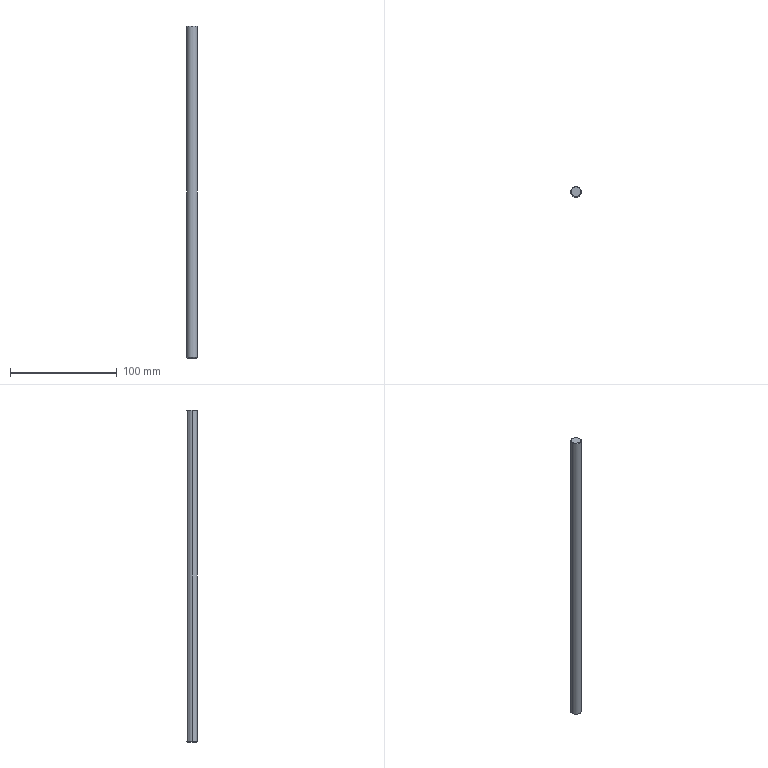Part | STEP file | PART2651.stp | 1 solid | 8 faces | box 10 x 10 x 311 mm | volume 24418 mm3 | cone 4 | plane 2 | cylinder 2 | commonest cylinder face diameters 10 x2
STEP:
#1=CARTESIAN_POINT('',(0.,0.,0.));
#2=DIRECTION('',(0.,0.,1.));
#3=DIRECTION('',(1.,0.,0.));
#4=AXIS2_PLACEMENT_3D('',#1,#2,#3);
#5=CARTESIAN_POINT('',(-5.,0.,410.5));
#6=VERTEX_POINT('',#5);
#7=CARTESIAN_POINT('',(-4.5,0.,411.));
#8=VERTEX_POINT('',#7);
#9=CARTESIAN_POINT('',(-5.,0.,410.5));
#10=DIRECTION('',(0.7071,0.,0.7071));
#11=VECTOR('',#10,1.);
#12=LINE('',#9,#11);
#13=CARTESIAN_POINT('',(0.,0.,411.025));
#14=DIRECTION('',(0.,0.,-1.));
#15=DIRECTION('',(-1.,0.,0.));
#16=AXIS2_PLACEMENT_3D('',#13,#14,#15);
#17=CONICAL_SURFACE('',#16,4.475,0.7854);
#18=CARTESIAN_POINT('',(0.,0.525));
#19=DIRECTION('',(0.,-1.));
#20=VECTOR('',#19,1.);
#21=LINE('',#18,#20);
#22=(GEOMETRIC_REPRESENTATION_CONTEXT(2)PARAMETRIC_REPRESENTATION_CONTEXT()REPRESENTATION_CONTEXT('',''));
#23=DEFINITIONAL_REPRESENTATION('',(#21),#22);
#24=PCURVE('',#17,#23);
#25=CARTESIAN_POINT('',(0.,0.,411.025));
#26=DIRECTION('',(0.,0.,-1.));
#27=DIRECTION('',(-1.,0.,0.));
#28=AXIS2_PLACEMENT_3D('',#25,#26,#27);
#29=CONICAL_SURFACE('',#28,4.475,0.7854);
#30=CARTESIAN_POINT('',(6.283,0.525));
#31=DIRECTION('',(0.,-1.));
#32=VECTOR('',#31,1.);
#33=LINE('',#30,#32);
#34=(GEOMETRIC_REPRESENTATION_CONTEXT(2)PARAMETRIC_REPRESENTATION_CONTEXT()REPRESENTATION_CONTEXT('',''));
#35=DEFINITIONAL_REPRESENTATION('',(#33),#34);
#36=PCURVE('',#29,#35);
#37=SURFACE_CURVE('',#12,(#24,#36),.PCURVE_S1.);
#38=EDGE_CURVE('',#6,#8,#37,.T.);
#39=ORIENTED_EDGE('',*,*,#38,.T.);
#40=CARTESIAN_POINT('',(4.5,0.,411.));
#41=VERTEX_POINT('',#40);
#42=CARTESIAN_POINT('',(0.,0.,411.));
#43=DIRECTION('',(0.,0.,1.));
#44=DIRECTION('',(1.,0.,0.));
#45=AXIS2_PLACEMENT_3D('',#42,#43,#44);
#46=CIRCLE('',#45,4.5);
#47=CARTESIAN_POINT('',(3.142,0.025));
#48=DIRECTION('',(-1.,0.));
#49=VECTOR('',#48,1.);
#50=LINE('',#47,#49);
#51=(GEOMETRIC_REPRESENTATION_CONTEXT(2)PARAMETRIC_REPRESENTATION_CONTEXT()REPRESENTATION_CONTEXT('',''));
#52=DEFINITIONAL_REPRESENTATION('',(#50),#51);
#53=PCURVE('',#17,#52);
#54=CARTESIAN_POINT('',(-4.95,-4.95,411.));
#55=DIRECTION('',(0.,0.,1.));
#56=DIRECTION('',(1.,0.,0.));
#57=AXIS2_PLACEMENT_3D('',#54,#55,#56);
#58=PLANE('',#57);
#59=CARTESIAN_POINT('',(4.95,4.95));
#60=DIRECTION('',(1.,0.));
#61=AXIS2_PLACEMENT_2D('',#59,#60);
#62=CIRCLE('',#61,4.5);
#63=(GEOMETRIC_REPRESENTATION_CONTEXT(2)PARAMETRIC_REPRESENTATION_CONTEXT()REPRESENTATION_CONTEXT('',''));
#64=DEFINITIONAL_REPRESENTATION('',(#62),#63);
#65=PCURVE('',#58,#64);
#66=SURFACE_CURVE('',#46,(#53,#65),.PCURVE_S1.);
#67=EDGE_CURVE('',#41,#8,#66,.T.);
#68=ORIENTED_EDGE('',*,*,#67,.F.);
#69=CARTESIAN_POINT('',(5.,0.,410.5));
#70=VERTEX_POINT('',#69);
#71=CARTESIAN_POINT('',(5.,0.,410.5));
#72=DIRECTION('',(-0.7071,0.,0.7071));
#73=VECTOR('',#72,1.);
#74=LINE('',#71,#73);
#75=CARTESIAN_POINT('',(3.142,0.525));
#76=DIRECTION('',(0.,-1.));
#77=VECTOR('',#76,1.);
#78=LINE('',#75,#77);
#79=(GEOMETRIC_REPRESENTATION_CONTEXT(2)PARAMETRIC_REPRESENTATION_CONTEXT()REPRESENTATION_CONTEXT('',''));
#80=DEFINITIONAL_REPRESENTATION('',(#78),#79);
#81=PCURVE('',#17,#80);
#82=CARTESIAN_POINT('',(3.142,0.525));
#83=DIRECTION('',(0.,-1.));
#84=VECTOR('',#83,1.);
#85=LINE('',#82,#84);
#86=(GEOMETRIC_REPRESENTATION_CONTEXT(2)PARAMETRIC_REPRESENTATION_CONTEXT()REPRESENTATION_CONTEXT('',''));
#87=DEFINITIONAL_REPRESENTATION('',(#85),#86);
#88=PCURVE('',#29,#87);
#89=SURFACE_CURVE('',#74,(#81,#88),.PCURVE_S1.);
#90=EDGE_CURVE('',#70,#41,#89,.T.);
#91=ORIENTED_EDGE('',*,*,#90,.F.);
#92=CARTESIAN_POINT('',(0.,0.,410.5));
#93=DIRECTION('',(0.,0.,-1.));
#94=DIRECTION('',(1.,0.,0.));
#95=AXIS2_PLACEMENT_3D('',#92,#93,#94);
#96=CIRCLE('',#95,5.);
#97=CARTESIAN_POINT('',(-3.142,0.525));
#98=DIRECTION('',(1.,0.));
#99=VECTOR('',#98,1.);
#100=LINE('',#97,#99);
#101=(GEOMETRIC_REPRESENTATION_CONTEXT(2)PARAMETRIC_REPRESENTATION_CONTEXT()REPRESENTATION_CONTEXT('',''));
#102=DEFINITIONAL_REPRESENTATION('',(#100),#101);
#103=PCURVE('',#17,#102);
#104=CARTESIAN_POINT('',(0.,0.,511.));
#105=DIRECTION('',(0.,0.,-1.));
#106=DIRECTION('',(-1.,0.,0.));
#107=AXIS2_PLACEMENT_3D('',#104,#105,#106);
#108=CYLINDRICAL_SURFACE('',#107,5.);
#109=CARTESIAN_POINT('',(-3.142,100.5));
#110=DIRECTION('',(1.,0.));
#111=VECTOR('',#110,1.);
#112=LINE('',#109,#111);
#113=(GEOMETRIC_REPRESENTATION_CONTEXT(2)PARAMETRIC_REPRESENTATION_CONTEXT()REPRESENTATION_CONTEXT('',''));
#114=DEFINITIONAL_REPRESENTATION('',(#112),#113);
#115=PCURVE('',#108,#114);
#116=SURFACE_CURVE('',#96,(#103,#115),.PCURVE_S1.);
#117=EDGE_CURVE('',#6,#70,#116,.T.);
#118=ORIENTED_EDGE('',*,*,#117,.F.);
#119=EDGE_LOOP('',(#39,#68,#91,#118));
#120=FACE_BOUND('',#119,.T.);
#121=ADVANCED_FACE('',(#120),#17,.T.);
#122=ORIENTED_EDGE('',*,*,#67,.T.);
#123=CARTESIAN_POINT('',(0.,0.,411.));
#124=DIRECTION('',(0.,0.,1.));
#125=DIRECTION('',(1.,0.,0.));
#126=AXIS2_PLACEMENT_3D('',#123,#124,#125);
#127=CIRCLE('',#126,4.5);
#128=CARTESIAN_POINT('',(4.95,4.95));
#129=DIRECTION('',(1.,0.));
#130=AXIS2_PLACEMENT_2D('',#128,#129);
#131=CIRCLE('',#130,4.5);
#132=(GEOMETRIC_REPRESENTATION_CONTEXT(2)PARAMETRIC_REPRESENTATION_CONTEXT()REPRESENTATION_CONTEXT('',''));
#133=DEFINITIONAL_REPRESENTATION('',(#131),#132);
#134=PCURVE('',#58,#133);
#135=CARTESIAN_POINT('',(9.425,0.025));
#136=DIRECTION('',(-1.,0.));
#137=VECTOR('',#136,1.);
#138=LINE('',#135,#137);
#139=(GEOMETRIC_REPRESENTATION_CONTEXT(2)PARAMETRIC_REPRESENTATION_CONTEXT()REPRESENTATION_CONTEXT('',''));
#140=DEFINITIONAL_REPRESENTATION('',(#138),#139);
#141=PCURVE('',#29,#140);
#142=SURFACE_CURVE('',#127,(#134,#141),.PCURVE_S1.);
#143=EDGE_CURVE('',#8,#41,#142,.T.);
#144=ORIENTED_EDGE('',*,*,#143,.T.);
#145=EDGE_LOOP('',(#122,#144));
#146=FACE_BOUND('',#145,.T.);
#147=ADVANCED_FACE('',(#146),#58,.T.);
#148=CARTESIAN_POINT('',(5.,0.,100.5));
#149=VERTEX_POINT('',#148);
#150=CARTESIAN_POINT('',(4.5,0.,100.));
#151=VERTEX_POINT('',#150);
#152=CARTESIAN_POINT('',(5.,0.,100.5));
#153=DIRECTION('',(-0.7071,0.,-0.7071));
#154=VECTOR('',#153,1.);
#155=LINE('',#152,#154);
#156=CARTESIAN_POINT('',(0.,0.,99.975));
#157=DIRECTION('',(0.,0.,1.));
#158=DIRECTION('',(1.,0.,0.));
#159=AXIS2_PLACEMENT_3D('',#156,#157,#158);
#160=CONICAL_SURFACE('',#159,4.475,0.7854);
#161=CARTESIAN_POINT('',(0.,0.525));
#162=DIRECTION('',(0.,-1.));
#163=VECTOR('',#162,1.);
#164=LINE('',#161,#163);
#165=(GEOMETRIC_REPRESENTATION_CONTEXT(2)PARAMETRIC_REPRESENTATION_CONTEXT()REPRESENTATION_CONTEXT('',''));
#166=DEFINITIONAL_REPRESENTATION('',(#164),#165);
#167=PCURVE('',#160,#166);
#168=CARTESIAN_POINT('',(0.,0.,99.975));
#169=DIRECTION('',(0.,0.,1.));
#170=DIRECTION('',(1.,0.,0.));
#171=AXIS2_PLACEMENT_3D('',#168,#169,#170);
#172=CONICAL_SURFACE('',#171,4.475,0.7854);
#173=CARTESIAN_POINT('',(6.283,0.525));
#174=DIRECTION('',(0.,-1.));
#175=VECTOR('',#174,1.);
#176=LINE('',#173,#175);
#177=(GEOMETRIC_REPRESENTATION_CONTEXT(2)PARAMETRIC_REPRESENTATION_CONTEXT()REPRESENTATION_CONTEXT('',''));
#178=DEFINITIONAL_REPRESENTATION('',(#176),#177);
#179=PCURVE('',#172,#178);
#180=SURFACE_CURVE('',#155,(#167,#179),.PCURVE_S1.);
#181=EDGE_CURVE('',#149,#151,#180,.T.);
#182=ORIENTED_EDGE('',*,*,#181,.T.);
#183=CARTESIAN_POINT('',(-4.5,0.,100.));
#184=VERTEX_POINT('',#183);
#185=CARTESIAN_POINT('',(0.,0.,100.));
#186=DIRECTION('',(0.,0.,-1.));
#187=DIRECTION('',(1.,0.,0.));
#188=AXIS2_PLACEMENT_3D('',#185,#186,#187);
#189=CIRCLE('',#188,4.5);
#190=CARTESIAN_POINT('',(6.283,0.025));
#191=DIRECTION('',(-1.,0.));
#192=VECTOR('',#191,1.);
#193=LINE('',#190,#192);
#194=(GEOMETRIC_REPRESENTATION_CONTEXT(2)PARAMETRIC_REPRESENTATION_CONTEXT()REPRESENTATION_CONTEXT('',''));
#195=DEFINITIONAL_REPRESENTATION('',(#193),#194);
#196=PCURVE('',#160,#195);
#197=CARTESIAN_POINT('',(-4.95,-4.95,100.));
#198=DIRECTION('',(0.,0.,1.));
#199=DIRECTION('',(1.,0.,0.));
#200=AXIS2_PLACEMENT_3D('',#197,#198,#199);
#201=PLANE('',#200);
#202=CARTESIAN_POINT('',(9.45,4.95));
#203=CARTESIAN_POINT('',(9.45,-2.844));
#204=CARTESIAN_POINT('',(2.7,1.053));
#205=CARTESIAN_POINT('',(-4.05,4.95));
#206=CARTESIAN_POINT('',(2.7,8.847));
#207=CARTESIAN_POINT('',(9.45,12.744));
#208=CARTESIAN_POINT('',(9.45,4.95));
#209=(BOUNDED_CURVE()B_SPLINE_CURVE(2,(#202,#203,#204,#205,#206,#207,#208),.UNSPECIFIED.,.T.,.F.)B_SPLINE_CURVE_WITH_KNOTS((1,2,2,2,2,1),(-2.094,0.,2.094,4.189,6.283,8.378),.UNSPECIFIED.)CURVE()GEOMETRIC_REPRESENTATION_ITEM()RATIONAL_B_SPLINE_CURVE((1.,0.5,1.,0.5,1.,0.5,1.))REPRESENTATION_ITEM(''));
#210=(GEOMETRIC_REPRESENTATION_CONTEXT(2)PARAMETRIC_REPRESENTATION_CONTEXT()REPRESENTATION_CONTEXT('',''));
#211=DEFINITIONAL_REPRESENTATION('',(#209),#210);
#212=PCURVE('',#201,#211);
#213=SURFACE_CURVE('',#189,(#196,#212),.PCURVE_S1.);
#214=EDGE_CURVE('',#184,#151,#213,.T.);
#215=ORIENTED_EDGE('',*,*,#214,.F.);
#216=CARTESIAN_POINT('',(-5.,0.,100.5));
#217=VERTEX_POINT('',#216);
#218=CARTESIAN_POINT('',(-5.,0.,100.5));
#219=DIRECTION('',(0.7071,0.,-0.7071));
#220=VECTOR('',#219,1.);
#221=LINE('',#218,#220);
#222=CARTESIAN_POINT('',(3.142,0.525));
#223=DIRECTION('',(0.,-1.));
#224=VECTOR('',#223,1.);
#225=LINE('',#222,#224);
#226=(GEOMETRIC_REPRESENTATION_CONTEXT(2)PARAMETRIC_REPRESENTATION_CONTEXT()REPRESENTATION_CONTEXT('',''));
#227=DEFINITIONAL_REPRESENTATION('',(#225),#226);
#228=PCURVE('',#160,#227);
#229=CARTESIAN_POINT('',(3.142,0.525));
#230=DIRECTION('',(0.,-1.));
#231=VECTOR('',#230,1.);
#232=LINE('',#229,#231);
#233=(GEOMETRIC_REPRESENTATION_CONTEXT(2)PARAMETRIC_REPRESENTATION_CONTEXT()REPRESENTATION_CONTEXT('',''));
#234=DEFINITIONAL_REPRESENTATION('',(#232),#233);
#235=PCURVE('',#172,#234);
#236=SURFACE_CURVE('',#221,(#228,#235),.PCURVE_S1.);
#237=EDGE_CURVE('',#217,#184,#236,.T.);
#238=ORIENTED_EDGE('',*,*,#237,.F.);
#239=CARTESIAN_POINT('',(0.,0.,100.5));
#240=DIRECTION('',(0.,0.,1.));
#241=DIRECTION('',(1.,0.,0.));
#242=AXIS2_PLACEMENT_3D('',#239,#240,#241);
#243=CIRCLE('',#242,5.);
#244=CARTESIAN_POINT('',(0.,0.525));
#245=DIRECTION('',(1.,0.));
#246=VECTOR('',#245,1.);
#247=LINE('',#244,#246);
#248=(GEOMETRIC_REPRESENTATION_CONTEXT(2)PARAMETRIC_REPRESENTATION_CONTEXT()REPRESENTATION_CONTEXT('',''));
#249=DEFINITIONAL_REPRESENTATION('',(#247),#248);
#250=PCURVE('',#160,#249);
#251=CARTESIAN_POINT('',(3.142,410.5));
#252=DIRECTION('',(-1.,0.));
#253=VECTOR('',#252,1.);
#254=LINE('',#251,#253);
#255=(GEOMETRIC_REPRESENTATION_CONTEXT(2)PARAMETRIC_REPRESENTATION_CONTEXT()REPRESENTATION_CONTEXT('',''));
#256=DEFINITIONAL_REPRESENTATION('',(#254),#255);
#257=PCURVE('',#108,#256);
#258=SURFACE_CURVE('',#243,(#250,#257),.PCURVE_S1.);
#259=EDGE_CURVE('',#149,#217,#258,.T.);
#260=ORIENTED_EDGE('',*,*,#259,.F.);
#261=EDGE_LOOP('',(#182,#215,#238,#260));
#262=FACE_BOUND('',#261,.T.);
#263=ADVANCED_FACE('',(#262),#160,.T.);
#264=CARTESIAN_POINT('',(0.,0.,100.));
#265=DIRECTION('',(0.,0.,-1.));
#266=DIRECTION('',(1.,0.,0.));
#267=AXIS2_PLACEMENT_3D('',#264,#265,#266);
#268=CIRCLE('',#267,4.5);
#269=CARTESIAN_POINT('',(9.45,4.95));
#270=CARTESIAN_POINT('',(9.45,-2.844));
#271=CARTESIAN_POINT('',(2.7,1.053));
#272=CARTESIAN_POINT('',(-4.05,4.95));
#273=CARTESIAN_POINT('',(2.7,8.847));
#274=CARTESIAN_POINT('',(9.45,12.744));
#275=CARTESIAN_POINT('',(9.45,4.95));
#276=(BOUNDED_CURVE()B_SPLINE_CURVE(2,(#269,#270,#271,#272,#273,#274,#275),.UNSPECIFIED.,.T.,.F.)B_SPLINE_CURVE_WITH_KNOTS((1,2,2,2,2,1),(-2.094,0.,2.094,4.189,6.283,8.378),.UNSPECIFIED.)CURVE()GEOMETRIC_REPRESENTATION_ITEM()RATIONAL_B_SPLINE_CURVE((1.,0.5,1.,0.5,1.,0.5,1.))REPRESENTATION_ITEM(''));
#277=(GEOMETRIC_REPRESENTATION_CONTEXT(2)PARAMETRIC_REPRESENTATION_CONTEXT()REPRESENTATION_CONTEXT('',''));
#278=DEFINITIONAL_REPRESENTATION('',(#276),#277);
#279=PCURVE('',#201,#278);
#280=CARTESIAN_POINT('',(6.283,0.025));
#281=DIRECTION('',(-1.,0.));
#282=VECTOR('',#281,1.);
#283=LINE('',#280,#282);
#284=(GEOMETRIC_REPRESENTATION_CONTEXT(2)PARAMETRIC_REPRESENTATION_CONTEXT()REPRESENTATION_CONTEXT('',''));
#285=DEFINITIONAL_REPRESENTATION('',(#283),#284);
#286=PCURVE('',#172,#285);
#287=SURFACE_CURVE('',#268,(#279,#286),.PCURVE_S1.);
#288=EDGE_CURVE('',#151,#184,#287,.T.);
#289=ORIENTED_EDGE('',*,*,#288,.T.);
#290=ORIENTED_EDGE('',*,*,#214,.T.);
#291=EDGE_LOOP('',(#289,#290));
#292=FACE_BOUND('',#291,.T.);
#293=ADVANCED_FACE('',(#292),#201,.F.);
#294=CARTESIAN_POINT('',(-5.,0.,100.5));
#295=DIRECTION('',(0.,0.,1.));
#296=VECTOR('',#295,1.);
#297=LINE('',#294,#296);
#298=CARTESIAN_POINT('',(0.,410.5));
#299=DIRECTION('',(0.,-1.));
#300=VECTOR('',#299,1.);
#301=LINE('',#298,#300);
#302=(GEOMETRIC_REPRESENTATION_CONTEXT(2)PARAMETRIC_REPRESENTATION_CONTEXT()REPRESENTATION_CONTEXT('',''));
#303=DEFINITIONAL_REPRESENTATION('',(#301),#302);
#304=PCURVE('',#108,#303);
#305=CARTESIAN_POINT('',(0.,0.,511.));
#306=DIRECTION('',(0.,0.,-1.));
#307=DIRECTION('',(-1.,0.,0.));
#308=AXIS2_PLACEMENT_3D('',#305,#306,#307);
#309=CYLINDRICAL_SURFACE('',#308,5.);
#310=CARTESIAN_POINT('',(6.283,410.5));
#311=DIRECTION('',(0.,-1.));
#312=VECTOR('',#311,1.);
#313=LINE('',#310,#312);
#314=(GEOMETRIC_REPRESENTATION_CONTEXT(2)PARAMETRIC_REPRESENTATION_CONTEXT()REPRESENTATION_CONTEXT('',''));
#315=DEFINITIONAL_REPRESENTATION('',(#313),#314);
#316=PCURVE('',#309,#315);
#317=SURFACE_CURVE('',#297,(#304,#316),.PCURVE_S1.);
#318=EDGE_CURVE('',#217,#6,#317,.T.);
#319=ORIENTED_EDGE('',*,*,#318,.T.);
#320=ORIENTED_EDGE('',*,*,#117,.T.);
#321=CARTESIAN_POINT('',(5.,0.,100.5));
#322=DIRECTION('',(0.,0.,1.));
#323=VECTOR('',#322,1.);
#324=LINE('',#321,#323);
#325=CARTESIAN_POINT('',(3.142,410.5));
#326=DIRECTION('',(0.,-1.));
#327=VECTOR('',#326,1.);
#328=LINE('',#325,#327);
#329=(GEOMETRIC_REPRESENTATION_CONTEXT(2)PARAMETRIC_REPRESENTATION_CONTEXT()REPRESENTATION_CONTEXT('',''));
#330=DEFINITIONAL_REPRESENTATION('',(#328),#329);
#331=PCURVE('',#108,#330);
#332=CARTESIAN_POINT('',(3.142,410.5));
#333=DIRECTION('',(0.,-1.));
#334=VECTOR('',#333,1.);
#335=LINE('',#332,#334);
#336=(GEOMETRIC_REPRESENTATION_CONTEXT(2)PARAMETRIC_REPRESENTATION_CONTEXT()REPRESENTATION_CONTEXT('',''));
#337=DEFINITIONAL_REPRESENTATION('',(#335),#336);
#338=PCURVE('',#309,#337);
#339=SURFACE_CURVE('',#324,(#331,#338),.PCURVE_S1.);
#340=EDGE_CURVE('',#149,#70,#339,.T.);
#341=ORIENTED_EDGE('',*,*,#340,.F.);
#342=ORIENTED_EDGE('',*,*,#259,.T.);
#343=EDGE_LOOP('',(#319,#320,#341,#342));
#344=FACE_BOUND('',#343,.T.);
#345=ADVANCED_FACE('',(#344),#108,.T.);
#346=ORIENTED_EDGE('',*,*,#318,.F.);
#347=CARTESIAN_POINT('',(0.,0.,100.5));
#348=DIRECTION('',(0.,0.,1.));
#349=DIRECTION('',(1.,0.,0.));
#350=AXIS2_PLACEMENT_3D('',#347,#348,#349);
#351=CIRCLE('',#350,5.);
#352=CARTESIAN_POINT('',(9.425,410.5));
#353=DIRECTION('',(-1.,0.));
#354=VECTOR('',#353,1.);
#355=LINE('',#352,#354);
#356=(GEOMETRIC_REPRESENTATION_CONTEXT(2)PARAMETRIC_REPRESENTATION_CONTEXT()REPRESENTATION_CONTEXT('',''));
#357=DEFINITIONAL_REPRESENTATION('',(#355),#356);
#358=PCURVE('',#309,#357);
#359=CARTESIAN_POINT('',(0.,0.525));
#360=DIRECTION('',(1.,0.));
#361=VECTOR('',#360,1.);
#362=LINE('',#359,#361);
#363=(GEOMETRIC_REPRESENTATION_CONTEXT(2)PARAMETRIC_REPRESENTATION_CONTEXT()REPRESENTATION_CONTEXT('',''));
#364=DEFINITIONAL_REPRESENTATION('',(#362),#363);
#365=PCURVE('',#172,#364);
#366=SURFACE_CURVE('',#351,(#358,#365),.PCURVE_S1.);
#367=EDGE_CURVE('',#217,#149,#366,.T.);
#368=ORIENTED_EDGE('',*,*,#367,.T.);
#369=ORIENTED_EDGE('',*,*,#340,.T.);
#370=CARTESIAN_POINT('',(0.,0.,410.5));
#371=DIRECTION('',(0.,0.,-1.));
#372=DIRECTION('',(1.,0.,0.));
#373=AXIS2_PLACEMENT_3D('',#370,#371,#372);
#374=CIRCLE('',#373,5.);
#375=CARTESIAN_POINT('',(3.142,100.5));
#376=DIRECTION('',(1.,0.));
#377=VECTOR('',#376,1.);
#378=LINE('',#375,#377);
#379=(GEOMETRIC_REPRESENTATION_CONTEXT(2)PARAMETRIC_REPRESENTATION_CONTEXT()REPRESENTATION_CONTEXT('',''));
#380=DEFINITIONAL_REPRESENTATION('',(#378),#379);
#381=PCURVE('',#309,#380);
#382=CARTESIAN_POINT('',(3.142,0.525));
#383=DIRECTION('',(1.,0.));
#384=VECTOR('',#383,1.);
#385=LINE('',#382,#384);
#386=(GEOMETRIC_REPRESENTATION_CONTEXT(2)PARAMETRIC_REPRESENTATION_CONTEXT()REPRESENTATION_CONTEXT('',''));
#387=DEFINITIONAL_REPRESENTATION('',(#385),#386);
#388=PCURVE('',#29,#387);
#389=SURFACE_CURVE('',#374,(#381,#388),.PCURVE_S1.);
#390=EDGE_CURVE('',#70,#6,#389,.T.);
#391=ORIENTED_EDGE('',*,*,#390,.T.);
#392=EDGE_LOOP('',(#346,#368,#369,#391));
#393=FACE_BOUND('',#392,.T.);
#394=ADVANCED_FACE('',(#393),#309,.T.);
#395=ORIENTED_EDGE('',*,*,#181,.F.);
#396=ORIENTED_EDGE('',*,*,#367,.F.);
#397=ORIENTED_EDGE('',*,*,#237,.T.);
#398=ORIENTED_EDGE('',*,*,#288,.F.);
#399=EDGE_LOOP('',(#395,#396,#397,#398));
#400=FACE_BOUND('',#399,.T.);
#401=ADVANCED_FACE('',(#400),#172,.T.);
#402=ORIENTED_EDGE('',*,*,#38,.F.);
#403=ORIENTED_EDGE('',*,*,#390,.F.);
#404=ORIENTED_EDGE('',*,*,#90,.T.);
#405=ORIENTED_EDGE('',*,*,#143,.F.);
#406=EDGE_LOOP('',(#402,#403,#404,#405));
#407=FACE_BOUND('',#406,.T.);
#408=ADVANCED_FACE('',(#407),#29,.T.);
#409=CLOSED_SHELL('',(#121,#147,#263,#293,#345,#394,#401,#408));
#410=MANIFOLD_SOLID_BREP('',#409);
#411=(LENGTH_UNIT()NAMED_UNIT(*)SI_UNIT(.MILLI.,.METRE.));
#412=UNCERTAINTY_MEASURE_WITH_UNIT(LENGTH_MEASURE(0.0000001),#411,'','');
#413=(NAMED_UNIT(*)PLANE_ANGLE_UNIT()SI_UNIT($,.RADIAN.));
#414=(NAMED_UNIT(*)SI_UNIT($,.STERADIAN.)SOLID_ANGLE_UNIT());
#415=(GEOMETRIC_REPRESENTATION_CONTEXT(3)GLOBAL_UNCERTAINTY_ASSIGNED_CONTEXT((#412))GLOBAL_UNIT_ASSIGNED_CONTEXT((#411,#413,#414))REPRESENTATION_CONTEXT('',''));
#416=ADVANCED_BREP_SHAPE_REPRESENTATION('',(#4,#410),#415);